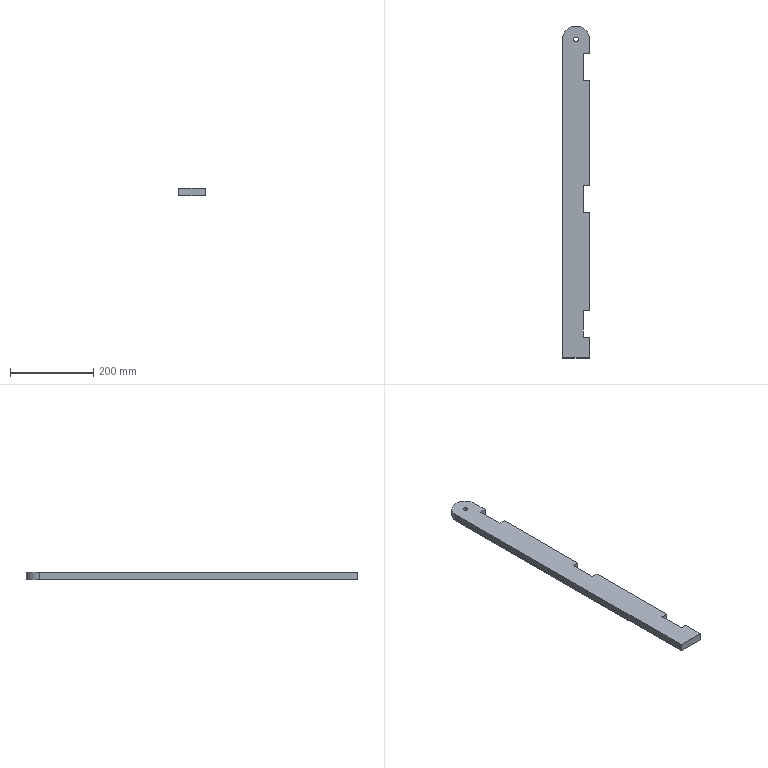Part | STEP file | Superstructure_3_1 | 1 solid | 19 faces | box 65 x 800 x 18 mm | volume 873479 mm3 | plane 17 | cylinder 2 | commonest cylinder face diameters 11 x1 65 x1
STEP:
#1=CARTESIAN_POINT('',(0.,0.,0.));
#2=DIRECTION('',(0.,0.,1.));
#3=DIRECTION('',(1.,0.,0.));
#4=AXIS2_PLACEMENT_3D('',#1,#2,#3);
#5=CARTESIAN_POINT('',(32.5,-35.,-9.));
#6=VERTEX_POINT('',#5);
#7=CARTESIAN_POINT('',(32.5,-35.,9.));
#8=VERTEX_POINT('',#7);
#9=CARTESIAN_POINT('',(32.5,-35.,-9.));
#10=DIRECTION('',(0.,0.,1.));
#11=VECTOR('',#10,1.);
#12=LINE('',#9,#11);
#13=CARTESIAN_POINT('',(32.5,-35.,-9.));
#14=DIRECTION('',(-1.,0.,0.));
#15=DIRECTION('',(0.,1.,0.));
#16=AXIS2_PLACEMENT_3D('',#13,#14,#15);
#17=PLANE('',#16);
#18=CARTESIAN_POINT('',(0.,0.));
#19=DIRECTION('',(0.,-1.));
#20=VECTOR('',#19,1.);
#21=LINE('',#18,#20);
#22=(GEOMETRIC_REPRESENTATION_CONTEXT(2)PARAMETRIC_REPRESENTATION_CONTEXT()REPRESENTATION_CONTEXT('',''));
#23=DEFINITIONAL_REPRESENTATION('',(#21),#22);
#24=PCURVE('',#17,#23);
#25=CARTESIAN_POINT('',(32.5,-35.,-9.));
#26=DIRECTION('',(0.,-1.,0.));
#27=DIRECTION('',(-1.,0.,0.));
#28=AXIS2_PLACEMENT_3D('',#25,#26,#27);
#29=PLANE('',#28);
#30=CARTESIAN_POINT('',(0.,0.));
#31=DIRECTION('',(0.,-1.));
#32=VECTOR('',#31,1.);
#33=LINE('',#30,#32);
#34=(GEOMETRIC_REPRESENTATION_CONTEXT(2)PARAMETRIC_REPRESENTATION_CONTEXT()REPRESENTATION_CONTEXT('',''));
#35=DEFINITIONAL_REPRESENTATION('',(#33),#34);
#36=PCURVE('',#29,#35);
#37=SURFACE_CURVE('',#12,(#24,#36),.PCURVE_S1.);
#38=EDGE_CURVE('',#6,#8,#37,.T.);
#39=ORIENTED_EDGE('',*,*,#38,.T.);
#40=CARTESIAN_POINT('',(32.5,0.,9.));
#41=VERTEX_POINT('',#40);
#42=CARTESIAN_POINT('',(32.5,-35.,9.));
#43=DIRECTION('',(0.,1.,0.));
#44=VECTOR('',#43,1.);
#45=LINE('',#42,#44);
#46=CARTESIAN_POINT('',(0.,-18.));
#47=DIRECTION('',(1.,0.));
#48=VECTOR('',#47,1.);
#49=LINE('',#46,#48);
#50=(GEOMETRIC_REPRESENTATION_CONTEXT(2)PARAMETRIC_REPRESENTATION_CONTEXT()REPRESENTATION_CONTEXT('',''));
#51=DEFINITIONAL_REPRESENTATION('',(#49),#50);
#52=PCURVE('',#17,#51);
#53=CARTESIAN_POINT('',(-0.3717,-369.588,9.));
#54=DIRECTION('',(0.,0.,1.));
#55=DIRECTION('',(1.,0.,0.));
#56=AXIS2_PLACEMENT_3D('',#53,#54,#55);
#57=PLANE('',#56);
#58=CARTESIAN_POINT('',(32.872,334.588));
#59=DIRECTION('',(0.,1.));
#60=VECTOR('',#59,1.);
#61=LINE('',#58,#60);
#62=(GEOMETRIC_REPRESENTATION_CONTEXT(2)PARAMETRIC_REPRESENTATION_CONTEXT()REPRESENTATION_CONTEXT('',''));
#63=DEFINITIONAL_REPRESENTATION('',(#61),#62);
#64=PCURVE('',#57,#63);
#65=SURFACE_CURVE('',#45,(#52,#64),.PCURVE_S1.);
#66=EDGE_CURVE('',#8,#41,#65,.T.);
#67=ORIENTED_EDGE('',*,*,#66,.T.);
#68=CARTESIAN_POINT('',(32.5,0.,-9.));
#69=VERTEX_POINT('',#68);
#70=CARTESIAN_POINT('',(32.5,0.,-9.));
#71=DIRECTION('',(0.,0.,1.));
#72=VECTOR('',#71,1.);
#73=LINE('',#70,#72);
#74=CARTESIAN_POINT('',(35.,0.));
#75=DIRECTION('',(0.,-1.));
#76=VECTOR('',#75,1.);
#77=LINE('',#74,#76);
#78=(GEOMETRIC_REPRESENTATION_CONTEXT(2)PARAMETRIC_REPRESENTATION_CONTEXT()REPRESENTATION_CONTEXT('',''));
#79=DEFINITIONAL_REPRESENTATION('',(#77),#78);
#80=PCURVE('',#17,#79);
#81=CARTESIAN_POINT('',(0.,0.,-9.));
#82=DIRECTION('',(0.,0.,-1.));
#83=DIRECTION('',(1.,0.,0.));
#84=AXIS2_PLACEMENT_3D('',#81,#82,#83);
#85=CYLINDRICAL_SURFACE('',#84,32.5);
#86=CARTESIAN_POINT('',(6.283,0.));
#87=DIRECTION('',(0.,-1.));
#88=VECTOR('',#87,1.);
#89=LINE('',#86,#88);
#90=(GEOMETRIC_REPRESENTATION_CONTEXT(2)PARAMETRIC_REPRESENTATION_CONTEXT()REPRESENTATION_CONTEXT('',''));
#91=DEFINITIONAL_REPRESENTATION('',(#89),#90);
#92=PCURVE('',#85,#91);
#93=SURFACE_CURVE('',#73,(#80,#92),.PCURVE_S1.);
#94=EDGE_CURVE('',#69,#41,#93,.T.);
#95=ORIENTED_EDGE('',*,*,#94,.F.);
#96=CARTESIAN_POINT('',(32.5,-35.,-9.));
#97=DIRECTION('',(0.,1.,0.));
#98=VECTOR('',#97,1.);
#99=LINE('',#96,#98);
#100=CARTESIAN_POINT('',(0.,0.));
#101=DIRECTION('',(1.,0.));
#102=VECTOR('',#101,1.);
#103=LINE('',#100,#102);
#104=(GEOMETRIC_REPRESENTATION_CONTEXT(2)PARAMETRIC_REPRESENTATION_CONTEXT()REPRESENTATION_CONTEXT('',''));
#105=DEFINITIONAL_REPRESENTATION('',(#103),#104);
#106=PCURVE('',#17,#105);
#107=CARTESIAN_POINT('',(-0.3717,-369.588,-9.));
#108=DIRECTION('',(0.,0.,1.));
#109=DIRECTION('',(1.,0.,0.));
#110=AXIS2_PLACEMENT_3D('',#107,#108,#109);
#111=PLANE('',#110);
#112=CARTESIAN_POINT('',(32.872,334.588));
#113=DIRECTION('',(0.,1.));
#114=VECTOR('',#113,1.);
#115=LINE('',#112,#114);
#116=(GEOMETRIC_REPRESENTATION_CONTEXT(2)PARAMETRIC_REPRESENTATION_CONTEXT()REPRESENTATION_CONTEXT('',''));
#117=DEFINITIONAL_REPRESENTATION('',(#115),#116);
#118=PCURVE('',#111,#117);
#119=SURFACE_CURVE('',#99,(#106,#118),.PCURVE_S1.);
#120=EDGE_CURVE('',#6,#69,#119,.T.);
#121=ORIENTED_EDGE('',*,*,#120,.F.);
#122=EDGE_LOOP('',(#39,#67,#95,#121));
#123=FACE_BOUND('',#122,.F.);
#124=ADVANCED_FACE('',(#123),#17,.F.);
#125=CARTESIAN_POINT('',(-32.5,0.,-9.));
#126=VERTEX_POINT('',#125);
#127=CARTESIAN_POINT('',(0.,0.,-9.));
#128=DIRECTION('',(0.,0.,1.));
#129=DIRECTION('',(1.,0.,0.));
#130=AXIS2_PLACEMENT_3D('',#127,#128,#129);
#131=CIRCLE('',#130,32.5);
#132=CARTESIAN_POINT('',(6.283,0.));
#133=DIRECTION('',(-1.,0.));
#134=VECTOR('',#133,1.);
#135=LINE('',#132,#134);
#136=(GEOMETRIC_REPRESENTATION_CONTEXT(2)PARAMETRIC_REPRESENTATION_CONTEXT()REPRESENTATION_CONTEXT('',''));
#137=DEFINITIONAL_REPRESENTATION('',(#135),#136);
#138=PCURVE('',#85,#137);
#139=CARTESIAN_POINT('',(0.3717,369.588));
#140=DIRECTION('',(1.,0.));
#141=AXIS2_PLACEMENT_2D('',#139,#140);
#142=CIRCLE('',#141,32.5);
#143=(GEOMETRIC_REPRESENTATION_CONTEXT(2)PARAMETRIC_REPRESENTATION_CONTEXT()REPRESENTATION_CONTEXT('',''));
#144=DEFINITIONAL_REPRESENTATION('',(#142),#143);
#145=PCURVE('',#111,#144);
#146=SURFACE_CURVE('',#131,(#138,#145),.PCURVE_S1.);
#147=EDGE_CURVE('',#69,#126,#146,.T.);
#148=ORIENTED_EDGE('',*,*,#147,.T.);
#149=CARTESIAN_POINT('',(-32.5,0.,9.));
#150=VERTEX_POINT('',#149);
#151=CARTESIAN_POINT('',(-32.5,0.,-9.));
#152=DIRECTION('',(0.,0.,1.));
#153=VECTOR('',#152,1.);
#154=LINE('',#151,#153);
#155=CARTESIAN_POINT('',(3.142,0.));
#156=DIRECTION('',(0.,-1.));
#157=VECTOR('',#156,1.);
#158=LINE('',#155,#157);
#159=(GEOMETRIC_REPRESENTATION_CONTEXT(2)PARAMETRIC_REPRESENTATION_CONTEXT()REPRESENTATION_CONTEXT('',''));
#160=DEFINITIONAL_REPRESENTATION('',(#158),#159);
#161=PCURVE('',#85,#160);
#162=CARTESIAN_POINT('',(-32.5,0.,-9.));
#163=DIRECTION('',(1.,0.,0.));
#164=DIRECTION('',(0.,-1.,0.));
#165=AXIS2_PLACEMENT_3D('',#162,#163,#164);
#166=PLANE('',#165);
#167=CARTESIAN_POINT('',(0.,0.));
#168=DIRECTION('',(0.,-1.));
#169=VECTOR('',#168,1.);
#170=LINE('',#167,#169);
#171=(GEOMETRIC_REPRESENTATION_CONTEXT(2)PARAMETRIC_REPRESENTATION_CONTEXT()REPRESENTATION_CONTEXT('',''));
#172=DEFINITIONAL_REPRESENTATION('',(#170),#171);
#173=PCURVE('',#166,#172);
#174=SURFACE_CURVE('',#154,(#161,#173),.PCURVE_S1.);
#175=EDGE_CURVE('',#126,#150,#174,.T.);
#176=ORIENTED_EDGE('',*,*,#175,.T.);
#177=CARTESIAN_POINT('',(0.,0.,9.));
#178=DIRECTION('',(0.,0.,1.));
#179=DIRECTION('',(1.,0.,0.));
#180=AXIS2_PLACEMENT_3D('',#177,#178,#179);
#181=CIRCLE('',#180,32.5);
#182=CARTESIAN_POINT('',(6.283,-18.));
#183=DIRECTION('',(-1.,0.));
#184=VECTOR('',#183,1.);
#185=LINE('',#182,#184);
#186=(GEOMETRIC_REPRESENTATION_CONTEXT(2)PARAMETRIC_REPRESENTATION_CONTEXT()REPRESENTATION_CONTEXT('',''));
#187=DEFINITIONAL_REPRESENTATION('',(#185),#186);
#188=PCURVE('',#85,#187);
#189=CARTESIAN_POINT('',(0.3717,369.588));
#190=DIRECTION('',(1.,0.));
#191=AXIS2_PLACEMENT_2D('',#189,#190);
#192=CIRCLE('',#191,32.5);
#193=(GEOMETRIC_REPRESENTATION_CONTEXT(2)PARAMETRIC_REPRESENTATION_CONTEXT()REPRESENTATION_CONTEXT('',''));
#194=DEFINITIONAL_REPRESENTATION('',(#192),#193);
#195=PCURVE('',#57,#194);
#196=SURFACE_CURVE('',#181,(#188,#195),.PCURVE_S1.);
#197=EDGE_CURVE('',#41,#150,#196,.T.);
#198=ORIENTED_EDGE('',*,*,#197,.F.);
#199=ORIENTED_EDGE('',*,*,#94,.F.);
#200=EDGE_LOOP('',(#148,#176,#198,#199));
#201=FACE_BOUND('',#200,.T.);
#202=ADVANCED_FACE('',(#201),#85,.T.);
#203=ORIENTED_EDGE('',*,*,#175,.T.);
#204=CARTESIAN_POINT('',(-32.5,-767.5,9.));
#205=VERTEX_POINT('',#204);
#206=CARTESIAN_POINT('',(-32.5,0.,9.));
#207=DIRECTION('',(0.,-1.,0.));
#208=VECTOR('',#207,1.);
#209=LINE('',#206,#208);
#210=CARTESIAN_POINT('',(0.,-18.));
#211=DIRECTION('',(1.,0.));
#212=VECTOR('',#211,1.);
#213=LINE('',#210,#212);
#214=(GEOMETRIC_REPRESENTATION_CONTEXT(2)PARAMETRIC_REPRESENTATION_CONTEXT()REPRESENTATION_CONTEXT('',''));
#215=DEFINITIONAL_REPRESENTATION('',(#213),#214);
#216=PCURVE('',#166,#215);
#217=CARTESIAN_POINT('',(-32.128,369.588));
#218=DIRECTION('',(0.,-1.));
#219=VECTOR('',#218,1.);
#220=LINE('',#217,#219);
#221=(GEOMETRIC_REPRESENTATION_CONTEXT(2)PARAMETRIC_REPRESENTATION_CONTEXT()REPRESENTATION_CONTEXT('',''));
#222=DEFINITIONAL_REPRESENTATION('',(#220),#221);
#223=PCURVE('',#57,#222);
#224=SURFACE_CURVE('',#209,(#216,#223),.PCURVE_S1.);
#225=EDGE_CURVE('',#150,#205,#224,.T.);
#226=ORIENTED_EDGE('',*,*,#225,.T.);
#227=CARTESIAN_POINT('',(-32.5,-767.5,-9.));
#228=VERTEX_POINT('',#227);
#229=CARTESIAN_POINT('',(-32.5,-767.5,-9.));
#230=DIRECTION('',(0.,0.,1.));
#231=VECTOR('',#230,1.);
#232=LINE('',#229,#231);
#233=CARTESIAN_POINT('',(767.5,0.));
#234=DIRECTION('',(0.,-1.));
#235=VECTOR('',#234,1.);
#236=LINE('',#233,#235);
#237=(GEOMETRIC_REPRESENTATION_CONTEXT(2)PARAMETRIC_REPRESENTATION_CONTEXT()REPRESENTATION_CONTEXT('',''));
#238=DEFINITIONAL_REPRESENTATION('',(#236),#237);
#239=PCURVE('',#166,#238);
#240=CARTESIAN_POINT('',(-32.5,-767.5,-9.));
#241=DIRECTION('',(0.,1.,0.));
#242=DIRECTION('',(1.,0.,0.));
#243=AXIS2_PLACEMENT_3D('',#240,#241,#242);
#244=PLANE('',#243);
#245=CARTESIAN_POINT('',(0.,0.));
#246=DIRECTION('',(0.,-1.));
#247=VECTOR('',#246,1.);
#248=LINE('',#245,#247);
#249=(GEOMETRIC_REPRESENTATION_CONTEXT(2)PARAMETRIC_REPRESENTATION_CONTEXT()REPRESENTATION_CONTEXT('',''));
#250=DEFINITIONAL_REPRESENTATION('',(#248),#249);
#251=PCURVE('',#244,#250);
#252=SURFACE_CURVE('',#232,(#239,#251),.PCURVE_S1.);
#253=EDGE_CURVE('',#228,#205,#252,.T.);
#254=ORIENTED_EDGE('',*,*,#253,.F.);
#255=CARTESIAN_POINT('',(-32.5,0.,-9.));
#256=DIRECTION('',(0.,-1.,0.));
#257=VECTOR('',#256,1.);
#258=LINE('',#255,#257);
#259=CARTESIAN_POINT('',(0.,0.));
#260=DIRECTION('',(1.,0.));
#261=VECTOR('',#260,1.);
#262=LINE('',#259,#261);
#263=(GEOMETRIC_REPRESENTATION_CONTEXT(2)PARAMETRIC_REPRESENTATION_CONTEXT()REPRESENTATION_CONTEXT('',''));
#264=DEFINITIONAL_REPRESENTATION('',(#262),#263);
#265=PCURVE('',#166,#264);
#266=CARTESIAN_POINT('',(-32.128,369.588));
#267=DIRECTION('',(0.,-1.));
#268=VECTOR('',#267,1.);
#269=LINE('',#266,#268);
#270=(GEOMETRIC_REPRESENTATION_CONTEXT(2)PARAMETRIC_REPRESENTATION_CONTEXT()REPRESENTATION_CONTEXT('',''));
#271=DEFINITIONAL_REPRESENTATION('',(#269),#270);
#272=PCURVE('',#111,#271);
#273=SURFACE_CURVE('',#258,(#265,#272),.PCURVE_S1.);
#274=EDGE_CURVE('',#126,#228,#273,.T.);
#275=ORIENTED_EDGE('',*,*,#274,.F.);
#276=EDGE_LOOP('',(#203,#226,#254,#275));
#277=FACE_BOUND('',#276,.F.);
#278=ADVANCED_FACE('',(#277),#166,.F.);
#279=ORIENTED_EDGE('',*,*,#253,.T.);
#280=CARTESIAN_POINT('',(32.5,-767.5,9.));
#281=VERTEX_POINT('',#280);
#282=CARTESIAN_POINT('',(-32.5,-767.5,9.));
#283=DIRECTION('',(1.,0.,0.));
#284=VECTOR('',#283,1.);
#285=LINE('',#282,#284);
#286=CARTESIAN_POINT('',(0.,-18.));
#287=DIRECTION('',(1.,0.));
#288=VECTOR('',#287,1.);
#289=LINE('',#286,#288);
#290=(GEOMETRIC_REPRESENTATION_CONTEXT(2)PARAMETRIC_REPRESENTATION_CONTEXT()REPRESENTATION_CONTEXT('',''));
#291=DEFINITIONAL_REPRESENTATION('',(#289),#290);
#292=PCURVE('',#244,#291);
#293=CARTESIAN_POINT('',(-32.128,-397.912));
#294=DIRECTION('',(1.,0.));
#295=VECTOR('',#294,1.);
#296=LINE('',#293,#295);
#297=(GEOMETRIC_REPRESENTATION_CONTEXT(2)PARAMETRIC_REPRESENTATION_CONTEXT()REPRESENTATION_CONTEXT('',''));
#298=DEFINITIONAL_REPRESENTATION('',(#296),#297);
#299=PCURVE('',#57,#298);
#300=SURFACE_CURVE('',#285,(#292,#299),.PCURVE_S1.);
#301=EDGE_CURVE('',#205,#281,#300,.T.);
#302=ORIENTED_EDGE('',*,*,#301,.T.);
#303=CARTESIAN_POINT('',(32.5,-767.5,-9.));
#304=VERTEX_POINT('',#303);
#305=CARTESIAN_POINT('',(32.5,-767.5,-9.));
#306=DIRECTION('',(0.,0.,1.));
#307=VECTOR('',#306,1.);
#308=LINE('',#305,#307);
#309=CARTESIAN_POINT('',(65.,0.));
#310=DIRECTION('',(0.,-1.));
#311=VECTOR('',#310,1.);
#312=LINE('',#309,#311);
#313=(GEOMETRIC_REPRESENTATION_CONTEXT(2)PARAMETRIC_REPRESENTATION_CONTEXT()REPRESENTATION_CONTEXT('',''));
#314=DEFINITIONAL_REPRESENTATION('',(#312),#313);
#315=PCURVE('',#244,#314);
#316=CARTESIAN_POINT('',(32.5,-767.5,-9.));
#317=DIRECTION('',(-1.,0.,0.));
#318=DIRECTION('',(0.,1.,0.));
#319=AXIS2_PLACEMENT_3D('',#316,#317,#318);
#320=PLANE('',#319);
#321=CARTESIAN_POINT('',(0.,0.));
#322=DIRECTION('',(0.,-1.));
#323=VECTOR('',#322,1.);
#324=LINE('',#321,#323);
#325=(GEOMETRIC_REPRESENTATION_CONTEXT(2)PARAMETRIC_REPRESENTATION_CONTEXT()REPRESENTATION_CONTEXT('',''));
#326=DEFINITIONAL_REPRESENTATION('',(#324),#325);
#327=PCURVE('',#320,#326);
#328=SURFACE_CURVE('',#308,(#315,#327),.PCURVE_S1.);
#329=EDGE_CURVE('',#304,#281,#328,.T.);
#330=ORIENTED_EDGE('',*,*,#329,.F.);
#331=CARTESIAN_POINT('',(-32.5,-767.5,-9.));
#332=DIRECTION('',(1.,0.,0.));
#333=VECTOR('',#332,1.);
#334=LINE('',#331,#333);
#335=CARTESIAN_POINT('',(0.,0.));
#336=DIRECTION('',(1.,0.));
#337=VECTOR('',#336,1.);
#338=LINE('',#335,#337);
#339=(GEOMETRIC_REPRESENTATION_CONTEXT(2)PARAMETRIC_REPRESENTATION_CONTEXT()REPRESENTATION_CONTEXT('',''));
#340=DEFINITIONAL_REPRESENTATION('',(#338),#339);
#341=PCURVE('',#244,#340);
#342=CARTESIAN_POINT('',(-32.128,-397.912));
#343=DIRECTION('',(1.,0.));
#344=VECTOR('',#343,1.);
#345=LINE('',#342,#344);
#346=(GEOMETRIC_REPRESENTATION_CONTEXT(2)PARAMETRIC_REPRESENTATION_CONTEXT()REPRESENTATION_CONTEXT('',''));
#347=DEFINITIONAL_REPRESENTATION('',(#345),#346);
#348=PCURVE('',#111,#347);
#349=SURFACE_CURVE('',#334,(#341,#348),.PCURVE_S1.);
#350=EDGE_CURVE('',#228,#304,#349,.T.);
#351=ORIENTED_EDGE('',*,*,#350,.F.);
#352=EDGE_LOOP('',(#279,#302,#330,#351));
#353=FACE_BOUND('',#352,.F.);
#354=ADVANCED_FACE('',(#353),#244,.F.);
#355=ORIENTED_EDGE('',*,*,#329,.T.);
#356=CARTESIAN_POINT('',(32.5,-717.5,9.));
#357=VERTEX_POINT('',#356);
#358=CARTESIAN_POINT('',(32.5,-767.5,9.));
#359=DIRECTION('',(0.,1.,0.));
#360=VECTOR('',#359,1.);
#361=LINE('',#358,#360);
#362=CARTESIAN_POINT('',(0.,-18.));
#363=DIRECTION('',(1.,0.));
#364=VECTOR('',#363,1.);
#365=LINE('',#362,#364);
#366=(GEOMETRIC_REPRESENTATION_CONTEXT(2)PARAMETRIC_REPRESENTATION_CONTEXT()REPRESENTATION_CONTEXT('',''));
#367=DEFINITIONAL_REPRESENTATION('',(#365),#366);
#368=PCURVE('',#320,#367);
#369=CARTESIAN_POINT('',(32.872,-397.912));
#370=DIRECTION('',(0.,1.));
#371=VECTOR('',#370,1.);
#372=LINE('',#369,#371);
#373=(GEOMETRIC_REPRESENTATION_CONTEXT(2)PARAMETRIC_REPRESENTATION_CONTEXT()REPRESENTATION_CONTEXT('',''));
#374=DEFINITIONAL_REPRESENTATION('',(#372),#373);
#375=PCURVE('',#57,#374);
#376=SURFACE_CURVE('',#361,(#368,#375),.PCURVE_S1.);
#377=EDGE_CURVE('',#281,#357,#376,.T.);
#378=ORIENTED_EDGE('',*,*,#377,.T.);
#379=CARTESIAN_POINT('',(32.5,-717.5,-9.));
#380=VERTEX_POINT('',#379);
#381=CARTESIAN_POINT('',(32.5,-717.5,-9.));
#382=DIRECTION('',(0.,0.,1.));
#383=VECTOR('',#382,1.);
#384=LINE('',#381,#383);
#385=CARTESIAN_POINT('',(50.,0.));
#386=DIRECTION('',(0.,-1.));
#387=VECTOR('',#386,1.);
#388=LINE('',#385,#387);
#389=(GEOMETRIC_REPRESENTATION_CONTEXT(2)PARAMETRIC_REPRESENTATION_CONTEXT()REPRESENTATION_CONTEXT('',''));
#390=DEFINITIONAL_REPRESENTATION('',(#388),#389);
#391=PCURVE('',#320,#390);
#392=CARTESIAN_POINT('',(32.5,-717.5,-9.));
#393=DIRECTION('',(0.,-1.,0.));
#394=DIRECTION('',(-1.,0.,0.));
#395=AXIS2_PLACEMENT_3D('',#392,#393,#394);
#396=PLANE('',#395);
#397=CARTESIAN_POINT('',(0.,0.));
#398=DIRECTION('',(0.,-1.));
#399=VECTOR('',#398,1.);
#400=LINE('',#397,#399);
#401=(GEOMETRIC_REPRESENTATION_CONTEXT(2)PARAMETRIC_REPRESENTATION_CONTEXT()REPRESENTATION_CONTEXT('',''));
#402=DEFINITIONAL_REPRESENTATION('',(#400),#401);
#403=PCURVE('',#396,#402);
#404=SURFACE_CURVE('',#384,(#391,#403),.PCURVE_S1.);
#405=EDGE_CURVE('',#380,#357,#404,.T.);
#406=ORIENTED_EDGE('',*,*,#405,.F.);
#407=CARTESIAN_POINT('',(32.5,-767.5,-9.));
#408=DIRECTION('',(0.,1.,0.));
#409=VECTOR('',#408,1.);
#410=LINE('',#407,#409);
#411=CARTESIAN_POINT('',(0.,0.));
#412=DIRECTION('',(1.,0.));
#413=VECTOR('',#412,1.);
#414=LINE('',#411,#413);
#415=(GEOMETRIC_REPRESENTATION_CONTEXT(2)PARAMETRIC_REPRESENTATION_CONTEXT()REPRESENTATION_CONTEXT('',''));
#416=DEFINITIONAL_REPRESENTATION('',(#414),#415);
#417=PCURVE('',#320,#416);
#418=CARTESIAN_POINT('',(32.872,-397.912));
#419=DIRECTION('',(0.,1.));
#420=VECTOR('',#419,1.);
#421=LINE('',#418,#420);
#422=(GEOMETRIC_REPRESENTATION_CONTEXT(2)PARAMETRIC_REPRESENTATION_CONTEXT()REPRESENTATION_CONTEXT('',''));
#423=DEFINITIONAL_REPRESENTATION('',(#421),#422);
#424=PCURVE('',#111,#423);
#425=SURFACE_CURVE('',#410,(#417,#424),.PCURVE_S1.);
#426=EDGE_CURVE('',#304,#380,#425,.T.);
#427=ORIENTED_EDGE('',*,*,#426,.F.);
#428=EDGE_LOOP('',(#355,#378,#406,#427));
#429=FACE_BOUND('',#428,.F.);
#430=ADVANCED_FACE('',(#429),#320,.F.);
#431=ORIENTED_EDGE('',*,*,#405,.T.);
#432=CARTESIAN_POINT('',(17.5,-717.5,9.));
#433=VERTEX_POINT('',#432);
#434=CARTESIAN_POINT('',(32.5,-717.5,9.));
#435=DIRECTION('',(-1.,0.,0.));
#436=VECTOR('',#435,1.);
#437=LINE('',#434,#436);
#438=CARTESIAN_POINT('',(0.,-18.));
#439=DIRECTION('',(1.,0.));
#440=VECTOR('',#439,1.);
#441=LINE('',#438,#440);
#442=(GEOMETRIC_REPRESENTATION_CONTEXT(2)PARAMETRIC_REPRESENTATION_CONTEXT()REPRESENTATION_CONTEXT('',''));
#443=DEFINITIONAL_REPRESENTATION('',(#441),#442);
#444=PCURVE('',#396,#443);
#445=CARTESIAN_POINT('',(32.872,-347.912));
#446=DIRECTION('',(-1.,0.));
#447=VECTOR('',#446,1.);
#448=LINE('',#445,#447);
#449=(GEOMETRIC_REPRESENTATION_CONTEXT(2)PARAMETRIC_REPRESENTATION_CONTEXT()REPRESENTATION_CONTEXT('',''));
#450=DEFINITIONAL_REPRESENTATION('',(#448),#449);
#451=PCURVE('',#57,#450);
#452=SURFACE_CURVE('',#437,(#444,#451),.PCURVE_S1.);
#453=EDGE_CURVE('',#357,#433,#452,.T.);
#454=ORIENTED_EDGE('',*,*,#453,.T.);
#455=CARTESIAN_POINT('',(17.5,-717.5,-9.));
#456=VERTEX_POINT('',#455);
#457=CARTESIAN_POINT('',(17.5,-717.5,-9.));
#458=DIRECTION('',(0.,0.,1.));
#459=VECTOR('',#458,1.);
#460=LINE('',#457,#459);
#461=CARTESIAN_POINT('',(15.,0.));
#462=DIRECTION('',(0.,-1.));
#463=VECTOR('',#462,1.);
#464=LINE('',#461,#463);
#465=(GEOMETRIC_REPRESENTATION_CONTEXT(2)PARAMETRIC_REPRESENTATION_CONTEXT()REPRESENTATION_CONTEXT('',''));
#466=DEFINITIONAL_REPRESENTATION('',(#464),#465);
#467=PCURVE('',#396,#466);
#468=CARTESIAN_POINT('',(17.5,-717.5,-9.));
#469=DIRECTION('',(-1.,0.,0.));
#470=DIRECTION('',(0.,1.,0.));
#471=AXIS2_PLACEMENT_3D('',#468,#469,#470);
#472=PLANE('',#471);
#473=CARTESIAN_POINT('',(0.,0.));
#474=DIRECTION('',(0.,-1.));
#475=VECTOR('',#474,1.);
#476=LINE('',#473,#475);
#477=(GEOMETRIC_REPRESENTATION_CONTEXT(2)PARAMETRIC_REPRESENTATION_CONTEXT()REPRESENTATION_CONTEXT('',''));
#478=DEFINITIONAL_REPRESENTATION('',(#476),#477);
#479=PCURVE('',#472,#478);
#480=SURFACE_CURVE('',#460,(#467,#479),.PCURVE_S1.);
#481=EDGE_CURVE('',#456,#433,#480,.T.);
#482=ORIENTED_EDGE('',*,*,#481,.F.);
#483=CARTESIAN_POINT('',(32.5,-717.5,-9.));
#484=DIRECTION('',(-1.,0.,0.));
#485=VECTOR('',#484,1.);
#486=LINE('',#483,#485);
#487=CARTESIAN_POINT('',(0.,0.));
#488=DIRECTION('',(1.,0.));
#489=VECTOR('',#488,1.);
#490=LINE('',#487,#489);
#491=(GEOMETRIC_REPRESENTATION_CONTEXT(2)PARAMETRIC_REPRESENTATION_CONTEXT()REPRESENTATION_CONTEXT('',''));
#492=DEFINITIONAL_REPRESENTATION('',(#490),#491);
#493=PCURVE('',#396,#492);
#494=CARTESIAN_POINT('',(32.872,-347.912));
#495=DIRECTION('',(-1.,0.));
#496=VECTOR('',#495,1.);
#497=LINE('',#494,#496);
#498=(GEOMETRIC_REPRESENTATION_CONTEXT(2)PARAMETRIC_REPRESENTATION_CONTEXT()REPRESENTATION_CONTEXT('',''));
#499=DEFINITIONAL_REPRESENTATION('',(#497),#498);
#500=PCURVE('',#111,#499);
#501=SURFACE_CURVE('',#486,(#493,#500),.PCURVE_S1.);
#502=EDGE_CURVE('',#380,#456,#501,.T.);
#503=ORIENTED_EDGE('',*,*,#502,.F.);
#504=EDGE_LOOP('',(#431,#454,#482,#503));
#505=FACE_BOUND('',#504,.F.);
#506=ADVANCED_FACE('',(#505),#396,.F.);
#507=ORIENTED_EDGE('',*,*,#481,.T.);
#508=CARTESIAN_POINT('',(17.5,-652.5,9.));
#509=VERTEX_POINT('',#508);
#510=CARTESIAN_POINT('',(17.5,-717.5,9.));
#511=DIRECTION('',(0.,1.,0.));
#512=VECTOR('',#511,1.);
#513=LINE('',#510,#512);
#514=CARTESIAN_POINT('',(0.,-18.));
#515=DIRECTION('',(1.,0.));
#516=VECTOR('',#515,1.);
#517=LINE('',#514,#516);
#518=(GEOMETRIC_REPRESENTATION_CONTEXT(2)PARAMETRIC_REPRESENTATION_CONTEXT()REPRESENTATION_CONTEXT('',''));
#519=DEFINITIONAL_REPRESENTATION('',(#517),#518);
#520=PCURVE('',#472,#519);
#521=CARTESIAN_POINT('',(17.872,-347.912));
#522=DIRECTION('',(0.,1.));
#523=VECTOR('',#522,1.);
#524=LINE('',#521,#523);
#525=(GEOMETRIC_REPRESENTATION_CONTEXT(2)PARAMETRIC_REPRESENTATION_CONTEXT()REPRESENTATION_CONTEXT('',''));
#526=DEFINITIONAL_REPRESENTATION('',(#524),#525);
#527=PCURVE('',#57,#526);
#528=SURFACE_CURVE('',#513,(#520,#527),.PCURVE_S1.);
#529=EDGE_CURVE('',#433,#509,#528,.T.);
#530=ORIENTED_EDGE('',*,*,#529,.T.);
#531=CARTESIAN_POINT('',(17.5,-652.5,-9.));
#532=VERTEX_POINT('',#531);
#533=CARTESIAN_POINT('',(17.5,-652.5,-9.));
#534=DIRECTION('',(0.,0.,1.));
#535=VECTOR('',#534,1.);
#536=LINE('',#533,#535);
#537=CARTESIAN_POINT('',(65.,0.));
#538=DIRECTION('',(0.,-1.));
#539=VECTOR('',#538,1.);
#540=LINE('',#537,#539);
#541=(GEOMETRIC_REPRESENTATION_CONTEXT(2)PARAMETRIC_REPRESENTATION_CONTEXT()REPRESENTATION_CONTEXT('',''));
#542=DEFINITIONAL_REPRESENTATION('',(#540),#541);
#543=PCURVE('',#472,#542);
#544=CARTESIAN_POINT('',(17.5,-652.5,-9.));
#545=DIRECTION('',(0.,1.,0.));
#546=DIRECTION('',(1.,0.,0.));
#547=AXIS2_PLACEMENT_3D('',#544,#545,#546);
#548=PLANE('',#547);
#549=CARTESIAN_POINT('',(0.,0.));
#550=DIRECTION('',(0.,-1.));
#551=VECTOR('',#550,1.);
#552=LINE('',#549,#551);
#553=(GEOMETRIC_REPRESENTATION_CONTEXT(2)PARAMETRIC_REPRESENTATION_CONTEXT()REPRESENTATION_CONTEXT('',''));
#554=DEFINITIONAL_REPRESENTATION('',(#552),#553);
#555=PCURVE('',#548,#554);
#556=SURFACE_CURVE('',#536,(#543,#555),.PCURVE_S1.);
#557=EDGE_CURVE('',#532,#509,#556,.T.);
#558=ORIENTED_EDGE('',*,*,#557,.F.);
#559=CARTESIAN_POINT('',(17.5,-717.5,-9.));
#560=DIRECTION('',(0.,1.,0.));
#561=VECTOR('',#560,1.);
#562=LINE('',#559,#561);
#563=CARTESIAN_POINT('',(0.,0.));
#564=DIRECTION('',(1.,0.));
#565=VECTOR('',#564,1.);
#566=LINE('',#563,#565);
#567=(GEOMETRIC_REPRESENTATION_CONTEXT(2)PARAMETRIC_REPRESENTATION_CONTEXT()REPRESENTATION_CONTEXT('',''));
#568=DEFINITIONAL_REPRESENTATION('',(#566),#567);
#569=PCURVE('',#472,#568);
#570=CARTESIAN_POINT('',(17.872,-347.912));
#571=DIRECTION('',(0.,1.));
#572=VECTOR('',#571,1.);
#573=LINE('',#570,#572);
#574=(GEOMETRIC_REPRESENTATION_CONTEXT(2)PARAMETRIC_REPRESENTATION_CONTEXT()REPRESENTATION_CONTEXT('',''));
#575=DEFINITIONAL_REPRESENTATION('',(#573),#574);
#576=PCURVE('',#111,#575);
#577=SURFACE_CURVE('',#562,(#569,#576),.PCURVE_S1.);
#578=EDGE_CURVE('',#456,#532,#577,.T.);
#579=ORIENTED_EDGE('',*,*,#578,.F.);
#580=EDGE_LOOP('',(#507,#530,#558,#579));
#581=FACE_BOUND('',#580,.F.);
#582=ADVANCED_FACE('',(#581),#472,.F.);
#583=ORIENTED_EDGE('',*,*,#557,.T.);
#584=CARTESIAN_POINT('',(32.5,-652.5,9.));
#585=VERTEX_POINT('',#584);
#586=CARTESIAN_POINT('',(17.5,-652.5,9.));
#587=DIRECTION('',(1.,0.,0.));
#588=VECTOR('',#587,1.);
#589=LINE('',#586,#588);
#590=CARTESIAN_POINT('',(0.,-18.));
#591=DIRECTION('',(1.,0.));
#592=VECTOR('',#591,1.);
#593=LINE('',#590,#592);
#594=(GEOMETRIC_REPRESENTATION_CONTEXT(2)PARAMETRIC_REPRESENTATION_CONTEXT()REPRESENTATION_CONTEXT('',''));
#595=DEFINITIONAL_REPRESENTATION('',(#593),#594);
#596=PCURVE('',#548,#595);
#597=CARTESIAN_POINT('',(17.872,-282.912));
#598=DIRECTION('',(1.,0.));
#599=VECTOR('',#598,1.);
#600=LINE('',#597,#599);
#601=(GEOMETRIC_REPRESENTATION_CONTEXT(2)PARAMETRIC_REPRESENTATION_CONTEXT()REPRESENTATION_CONTEXT('',''));
#602=DEFINITIONAL_REPRESENTATION('',(#600),#601);
#603=PCURVE('',#57,#602);
#604=SURFACE_CURVE('',#589,(#596,#603),.PCURVE_S1.);
#605=EDGE_CURVE('',#509,#585,#604,.T.);
#606=ORIENTED_EDGE('',*,*,#605,.T.);
#607=CARTESIAN_POINT('',(32.5,-652.5,-9.));
#608=VERTEX_POINT('',#607);
#609=CARTESIAN_POINT('',(32.5,-652.5,-9.));
#610=DIRECTION('',(0.,0.,1.));
#611=VECTOR('',#610,1.);
#612=LINE('',#609,#611);
#613=CARTESIAN_POINT('',(15.,0.));
#614=DIRECTION('',(0.,-1.));
#615=VECTOR('',#614,1.);
#616=LINE('',#613,#615);
#617=(GEOMETRIC_REPRESENTATION_CONTEXT(2)PARAMETRIC_REPRESENTATION_CONTEXT()REPRESENTATION_CONTEXT('',''));
#618=DEFINITIONAL_REPRESENTATION('',(#616),#617);
#619=PCURVE('',#548,#618);
#620=CARTESIAN_POINT('',(32.5,-652.5,-9.));
#621=DIRECTION('',(-1.,0.,0.));
#622=DIRECTION('',(0.,1.,0.));
#623=AXIS2_PLACEMENT_3D('',#620,#621,#622);
#624=PLANE('',#623);
#625=CARTESIAN_POINT('',(0.,0.));
#626=DIRECTION('',(0.,-1.));
#627=VECTOR('',#626,1.);
#628=LINE('',#625,#627);
#629=(GEOMETRIC_REPRESENTATION_CONTEXT(2)PARAMETRIC_REPRESENTATION_CONTEXT()REPRESENTATION_CONTEXT('',''));
#630=DEFINITIONAL_REPRESENTATION('',(#628),#629);
#631=PCURVE('',#624,#630);
#632=SURFACE_CURVE('',#612,(#619,#631),.PCURVE_S1.);
#633=EDGE_CURVE('',#608,#585,#632,.T.);
#634=ORIENTED_EDGE('',*,*,#633,.F.);
#635=CARTESIAN_POINT('',(17.5,-652.5,-9.));
#636=DIRECTION('',(1.,0.,0.));
#637=VECTOR('',#636,1.);
#638=LINE('',#635,#637);
#639=CARTESIAN_POINT('',(0.,0.));
#640=DIRECTION('',(1.,0.));
#641=VECTOR('',#640,1.);
#642=LINE('',#639,#641);
#643=(GEOMETRIC_REPRESENTATION_CONTEXT(2)PARAMETRIC_REPRESENTATION_CONTEXT()REPRESENTATION_CONTEXT('',''));
#644=DEFINITIONAL_REPRESENTATION('',(#642),#643);
#645=PCURVE('',#548,#644);
#646=CARTESIAN_POINT('',(17.872,-282.912));
#647=DIRECTION('',(1.,0.));
#648=VECTOR('',#647,1.);
#649=LINE('',#646,#648);
#650=(GEOMETRIC_REPRESENTATION_CONTEXT(2)PARAMETRIC_REPRESENTATION_CONTEXT()REPRESENTATION_CONTEXT('',''));
#651=DEFINITIONAL_REPRESENTATION('',(#649),#650);
#652=PCURVE('',#111,#651);
#653=SURFACE_CURVE('',#638,(#645,#652),.PCURVE_S1.);
#654=EDGE_CURVE('',#532,#608,#653,.T.);
#655=ORIENTED_EDGE('',*,*,#654,.F.);
#656=EDGE_LOOP('',(#583,#606,#634,#655));
#657=FACE_BOUND('',#656,.F.);
#658=ADVANCED_FACE('',(#657),#548,.F.);
#659=ORIENTED_EDGE('',*,*,#633,.T.);
#660=CARTESIAN_POINT('',(32.5,-416.25,9.));
#661=VERTEX_POINT('',#660);
#662=CARTESIAN_POINT('',(32.5,-652.5,9.));
#663=DIRECTION('',(0.,1.,0.));
#664=VECTOR('',#663,1.);
#665=LINE('',#662,#664);
#666=CARTESIAN_POINT('',(0.,-18.));
#667=DIRECTION('',(1.,0.));
#668=VECTOR('',#667,1.);
#669=LINE('',#666,#668);
#670=(GEOMETRIC_REPRESENTATION_CONTEXT(2)PARAMETRIC_REPRESENTATION_CONTEXT()REPRESENTATION_CONTEXT('',''));
#671=DEFINITIONAL_REPRESENTATION('',(#669),#670);
#672=PCURVE('',#624,#671);
#673=CARTESIAN_POINT('',(32.872,-282.912));
#674=DIRECTION('',(0.,1.));
#675=VECTOR('',#674,1.);
#676=LINE('',#673,#675);
#677=(GEOMETRIC_REPRESENTATION_CONTEXT(2)PARAMETRIC_REPRESENTATION_CONTEXT()REPRESENTATION_CONTEXT('',''));
#678=DEFINITIONAL_REPRESENTATION('',(#676),#677);
#679=PCURVE('',#57,#678);
#680=SURFACE_CURVE('',#665,(#672,#679),.PCURVE_S1.);
#681=EDGE_CURVE('',#585,#661,#680,.T.);
#682=ORIENTED_EDGE('',*,*,#681,.T.);
#683=CARTESIAN_POINT('',(32.5,-416.25,-9.));
#684=VERTEX_POINT('',#683);
#685=CARTESIAN_POINT('',(32.5,-416.25,-9.));
#686=DIRECTION('',(0.,0.,1.));
#687=VECTOR('',#686,1.);
#688=LINE('',#685,#687);
#689=CARTESIAN_POINT('',(236.25,0.));
#690=DIRECTION('',(0.,-1.));
#691=VECTOR('',#690,1.);
#692=LINE('',#689,#691);
#693=(GEOMETRIC_REPRESENTATION_CONTEXT(2)PARAMETRIC_REPRESENTATION_CONTEXT()REPRESENTATION_CONTEXT('',''));
#694=DEFINITIONAL_REPRESENTATION('',(#692),#693);
#695=PCURVE('',#624,#694);
#696=CARTESIAN_POINT('',(17.5,-416.25,-9.));
#697=DIRECTION('',(0.,1.,0.));
#698=DIRECTION('',(1.,0.,0.));
#699=AXIS2_PLACEMENT_3D('',#696,#697,#698);
#700=PLANE('',#699);
#701=CARTESIAN_POINT('',(15.,0.));
#702=DIRECTION('',(0.,-1.));
#703=VECTOR('',#702,1.);
#704=LINE('',#701,#703);
#705=(GEOMETRIC_REPRESENTATION_CONTEXT(2)PARAMETRIC_REPRESENTATION_CONTEXT()REPRESENTATION_CONTEXT('',''));
#706=DEFINITIONAL_REPRESENTATION('',(#704),#705);
#707=PCURVE('',#700,#706);
#708=SURFACE_CURVE('',#688,(#695,#707),.PCURVE_S1.);
#709=EDGE_CURVE('',#684,#661,#708,.T.);
#710=ORIENTED_EDGE('',*,*,#709,.F.);
#711=CARTESIAN_POINT('',(32.5,-652.5,-9.));
#712=DIRECTION('',(0.,1.,0.));
#713=VECTOR('',#712,1.);
#714=LINE('',#711,#713);
#715=CARTESIAN_POINT('',(0.,0.));
#716=DIRECTION('',(1.,0.));
#717=VECTOR('',#716,1.);
#718=LINE('',#715,#717);
#719=(GEOMETRIC_REPRESENTATION_CONTEXT(2)PARAMETRIC_REPRESENTATION_CONTEXT()REPRESENTATION_CONTEXT('',''));
#720=DEFINITIONAL_REPRESENTATION('',(#718),#719);
#721=PCURVE('',#624,#720);
#722=CARTESIAN_POINT('',(32.872,-282.912));
#723=DIRECTION('',(0.,1.));
#724=VECTOR('',#723,1.);
#725=LINE('',#722,#724);
#726=(GEOMETRIC_REPRESENTATION_CONTEXT(2)PARAMETRIC_REPRESENTATION_CONTEXT()REPRESENTATION_CONTEXT('',''));
#727=DEFINITIONAL_REPRESENTATION('',(#725),#726);
#728=PCURVE('',#111,#727);
#729=SURFACE_CURVE('',#714,(#721,#728),.PCURVE_S1.);
#730=EDGE_CURVE('',#608,#684,#729,.T.);
#731=ORIENTED_EDGE('',*,*,#730,.F.);
#732=EDGE_LOOP('',(#659,#682,#710,#731));
#733=FACE_BOUND('',#732,.F.);
#734=ADVANCED_FACE('',(#733),#624,.F.);
#735=CARTESIAN_POINT('',(17.5,-416.25,-9.));
#736=VERTEX_POINT('',#735);
#737=CARTESIAN_POINT('',(17.5,-416.25,9.));
#738=VERTEX_POINT('',#737);
#739=CARTESIAN_POINT('',(17.5,-416.25,-9.));
#740=DIRECTION('',(0.,0.,1.));
#741=VECTOR('',#740,1.);
#742=LINE('',#739,#741);
#743=CARTESIAN_POINT('',(0.,0.));
#744=DIRECTION('',(0.,-1.));
#745=VECTOR('',#744,1.);
#746=LINE('',#743,#745);
#747=(GEOMETRIC_REPRESENTATION_CONTEXT(2)PARAMETRIC_REPRESENTATION_CONTEXT()REPRESENTATION_CONTEXT('',''));
#748=DEFINITIONAL_REPRESENTATION('',(#746),#747);
#749=PCURVE('',#700,#748);
#750=CARTESIAN_POINT('',(17.5,-351.25,-9.));
#751=DIRECTION('',(1.,0.,0.));
#752=DIRECTION('',(0.,-1.,0.));
#753=AXIS2_PLACEMENT_3D('',#750,#751,#752);
#754=PLANE('',#753);
#755=CARTESIAN_POINT('',(65.,0.));
#756=DIRECTION('',(0.,-1.));
#757=VECTOR('',#756,1.);
#758=LINE('',#755,#757);
#759=(GEOMETRIC_REPRESENTATION_CONTEXT(2)PARAMETRIC_REPRESENTATION_CONTEXT()REPRESENTATION_CONTEXT('',''));
#760=DEFINITIONAL_REPRESENTATION('',(#758),#759);
#761=PCURVE('',#754,#760);
#762=SURFACE_CURVE('',#742,(#749,#761),.PCURVE_S1.);
#763=EDGE_CURVE('',#736,#738,#762,.T.);
#764=ORIENTED_EDGE('',*,*,#763,.T.);
#765=CARTESIAN_POINT('',(17.5,-416.25,9.));
#766=DIRECTION('',(1.,0.,0.));
#767=VECTOR('',#766,1.);
#768=LINE('',#765,#767);
#769=CARTESIAN_POINT('',(0.,-18.));
#770=DIRECTION('',(1.,0.));
#771=VECTOR('',#770,1.);
#772=LINE('',#769,#771);
#773=(GEOMETRIC_REPRESENTATION_CONTEXT(2)PARAMETRIC_REPRESENTATION_CONTEXT()REPRESENTATION_CONTEXT('',''));
#774=DEFINITIONAL_REPRESENTATION('',(#772),#773);
#775=PCURVE('',#700,#774);
#776=CARTESIAN_POINT('',(17.872,-46.662));
#777=DIRECTION('',(1.,0.));
#778=VECTOR('',#777,1.);
#779=LINE('',#776,#778);
#780=(GEOMETRIC_REPRESENTATION_CONTEXT(2)PARAMETRIC_REPRESENTATION_CONTEXT()REPRESENTATION_CONTEXT('',''));
#781=DEFINITIONAL_REPRESENTATION('',(#779),#780);
#782=PCURVE('',#57,#781);
#783=SURFACE_CURVE('',#768,(#775,#782),.PCURVE_S1.);
#784=EDGE_CURVE('',#738,#661,#783,.T.);
#785=ORIENTED_EDGE('',*,*,#784,.T.);
#786=ORIENTED_EDGE('',*,*,#709,.F.);
#787=CARTESIAN_POINT('',(17.5,-416.25,-9.));
#788=DIRECTION('',(1.,0.,0.));
#789=VECTOR('',#788,1.);
#790=LINE('',#787,#789);
#791=CARTESIAN_POINT('',(0.,0.));
#792=DIRECTION('',(1.,0.));
#793=VECTOR('',#792,1.);
#794=LINE('',#791,#793);
#795=(GEOMETRIC_REPRESENTATION_CONTEXT(2)PARAMETRIC_REPRESENTATION_CONTEXT()REPRESENTATION_CONTEXT('',''));
#796=DEFINITIONAL_REPRESENTATION('',(#794),#795);
#797=PCURVE('',#700,#796);
#798=CARTESIAN_POINT('',(17.872,-46.662));
#799=DIRECTION('',(1.,0.));
#800=VECTOR('',#799,1.);
#801=LINE('',#798,#800);
#802=(GEOMETRIC_REPRESENTATION_CONTEXT(2)PARAMETRIC_REPRESENTATION_CONTEXT()REPRESENTATION_CONTEXT('',''));
#803=DEFINITIONAL_REPRESENTATION('',(#801),#802);
#804=PCURVE('',#111,#803);
#805=SURFACE_CURVE('',#790,(#797,#804),.PCURVE_S1.);
#806=EDGE_CURVE('',#736,#684,#805,.T.);
#807=ORIENTED_EDGE('',*,*,#806,.F.);
#808=EDGE_LOOP('',(#764,#785,#786,#807));
#809=FACE_BOUND('',#808,.T.);
#810=ADVANCED_FACE('',(#809),#700,.T.);
#811=CARTESIAN_POINT('',(17.5,-351.25,-9.));
#812=VERTEX_POINT('',#811);
#813=CARTESIAN_POINT('',(17.5,-351.25,9.));
#814=VERTEX_POINT('',#813);
#815=CARTESIAN_POINT('',(17.5,-351.25,-9.));
#816=DIRECTION('',(0.,0.,1.));
#817=VECTOR('',#816,1.);
#818=LINE('',#815,#817);
#819=CARTESIAN_POINT('',(0.,0.));
#820=DIRECTION('',(0.,-1.));
#821=VECTOR('',#820,1.);
#822=LINE('',#819,#821);
#823=(GEOMETRIC_REPRESENTATION_CONTEXT(2)PARAMETRIC_REPRESENTATION_CONTEXT()REPRESENTATION_CONTEXT('',''));
#824=DEFINITIONAL_REPRESENTATION('',(#822),#823);
#825=PCURVE('',#754,#824);
#826=CARTESIAN_POINT('',(32.5,-351.25,-9.));
#827=DIRECTION('',(0.,-1.,0.));
#828=DIRECTION('',(-1.,0.,0.));
#829=AXIS2_PLACEMENT_3D('',#826,#827,#828);
#830=PLANE('',#829);
#831=CARTESIAN_POINT('',(15.,0.));
#832=DIRECTION('',(0.,-1.));
#833=VECTOR('',#832,1.);
#834=LINE('',#831,#833);
#835=(GEOMETRIC_REPRESENTATION_CONTEXT(2)PARAMETRIC_REPRESENTATION_CONTEXT()REPRESENTATION_CONTEXT('',''));
#836=DEFINITIONAL_REPRESENTATION('',(#834),#835);
#837=PCURVE('',#830,#836);
#838=SURFACE_CURVE('',#818,(#825,#837),.PCURVE_S1.);
#839=EDGE_CURVE('',#812,#814,#838,.T.);
#840=ORIENTED_EDGE('',*,*,#839,.T.);
#841=CARTESIAN_POINT('',(17.5,-351.25,9.));
#842=DIRECTION('',(0.,-1.,0.));
#843=VECTOR('',#842,1.);
#844=LINE('',#841,#843);
#845=CARTESIAN_POINT('',(0.,-18.));
#846=DIRECTION('',(1.,0.));
#847=VECTOR('',#846,1.);
#848=LINE('',#845,#847);
#849=(GEOMETRIC_REPRESENTATION_CONTEXT(2)PARAMETRIC_REPRESENTATION_CONTEXT()REPRESENTATION_CONTEXT('',''));
#850=DEFINITIONAL_REPRESENTATION('',(#848),#849);
#851=PCURVE('',#754,#850);
#852=CARTESIAN_POINT('',(17.872,18.338));
#853=DIRECTION('',(0.,-1.));
#854=VECTOR('',#853,1.);
#855=LINE('',#852,#854);
#856=(GEOMETRIC_REPRESENTATION_CONTEXT(2)PARAMETRIC_REPRESENTATION_CONTEXT()REPRESENTATION_CONTEXT('',''));
#857=DEFINITIONAL_REPRESENTATION('',(#855),#856);
#858=PCURVE('',#57,#857);
#859=SURFACE_CURVE('',#844,(#851,#858),.PCURVE_S1.);
#860=EDGE_CURVE('',#814,#738,#859,.T.);
#861=ORIENTED_EDGE('',*,*,#860,.T.);
#862=ORIENTED_EDGE('',*,*,#763,.F.);
#863=CARTESIAN_POINT('',(17.5,-351.25,-9.));
#864=DIRECTION('',(0.,-1.,0.));
#865=VECTOR('',#864,1.);
#866=LINE('',#863,#865);
#867=CARTESIAN_POINT('',(0.,0.));
#868=DIRECTION('',(1.,0.));
#869=VECTOR('',#868,1.);
#870=LINE('',#867,#869);
#871=(GEOMETRIC_REPRESENTATION_CONTEXT(2)PARAMETRIC_REPRESENTATION_CONTEXT()REPRESENTATION_CONTEXT('',''));
#872=DEFINITIONAL_REPRESENTATION('',(#870),#871);
#873=PCURVE('',#754,#872);
#874=CARTESIAN_POINT('',(17.872,18.338));
#875=DIRECTION('',(0.,-1.));
#876=VECTOR('',#875,1.);
#877=LINE('',#874,#876);
#878=(GEOMETRIC_REPRESENTATION_CONTEXT(2)PARAMETRIC_REPRESENTATION_CONTEXT()REPRESENTATION_CONTEXT('',''));
#879=DEFINITIONAL_REPRESENTATION('',(#877),#878);
#880=PCURVE('',#111,#879);
#881=SURFACE_CURVE('',#866,(#873,#880),.PCURVE_S1.);
#882=EDGE_CURVE('',#812,#736,#881,.T.);
#883=ORIENTED_EDGE('',*,*,#882,.F.);
#884=EDGE_LOOP('',(#840,#861,#862,#883));
#885=FACE_BOUND('',#884,.T.);
#886=ADVANCED_FACE('',(#885),#754,.T.);
#887=CARTESIAN_POINT('',(32.5,-351.25,-9.));
#888=VERTEX_POINT('',#887);
#889=CARTESIAN_POINT('',(32.5,-351.25,9.));
#890=VERTEX_POINT('',#889);
#891=CARTESIAN_POINT('',(32.5,-351.25,-9.));
#892=DIRECTION('',(0.,0.,1.));
#893=VECTOR('',#892,1.);
#894=LINE('',#891,#893);
#895=CARTESIAN_POINT('',(0.,0.));
#896=DIRECTION('',(0.,-1.));
#897=VECTOR('',#896,1.);
#898=LINE('',#895,#897);
#899=(GEOMETRIC_REPRESENTATION_CONTEXT(2)PARAMETRIC_REPRESENTATION_CONTEXT()REPRESENTATION_CONTEXT('',''));
#900=DEFINITIONAL_REPRESENTATION('',(#898),#899);
#901=PCURVE('',#830,#900);
#902=CARTESIAN_POINT('',(32.5,-351.25,-9.));
#903=DIRECTION('',(-1.,0.,0.));
#904=DIRECTION('',(0.,1.,0.));
#905=AXIS2_PLACEMENT_3D('',#902,#903,#904);
#906=PLANE('',#905);
#907=CARTESIAN_POINT('',(0.,0.));
#908=DIRECTION('',(0.,-1.));
#909=VECTOR('',#908,1.);
#910=LINE('',#907,#909);
#911=(GEOMETRIC_REPRESENTATION_CONTEXT(2)PARAMETRIC_REPRESENTATION_CONTEXT()REPRESENTATION_CONTEXT('',''));
#912=DEFINITIONAL_REPRESENTATION('',(#910),#911);
#913=PCURVE('',#906,#912);
#914=SURFACE_CURVE('',#894,(#901,#913),.PCURVE_S1.);
#915=EDGE_CURVE('',#888,#890,#914,.T.);
#916=ORIENTED_EDGE('',*,*,#915,.T.);
#917=CARTESIAN_POINT('',(32.5,-351.25,9.));
#918=DIRECTION('',(-1.,0.,0.));
#919=VECTOR('',#918,1.);
#920=LINE('',#917,#919);
#921=CARTESIAN_POINT('',(0.,-18.));
#922=DIRECTION('',(1.,0.));
#923=VECTOR('',#922,1.);
#924=LINE('',#921,#923);
#925=(GEOMETRIC_REPRESENTATION_CONTEXT(2)PARAMETRIC_REPRESENTATION_CONTEXT()REPRESENTATION_CONTEXT('',''));
#926=DEFINITIONAL_REPRESENTATION('',(#924),#925);
#927=PCURVE('',#830,#926);
#928=CARTESIAN_POINT('',(32.872,18.338));
#929=DIRECTION('',(-1.,0.));
#930=VECTOR('',#929,1.);
#931=LINE('',#928,#930);
#932=(GEOMETRIC_REPRESENTATION_CONTEXT(2)PARAMETRIC_REPRESENTATION_CONTEXT()REPRESENTATION_CONTEXT('',''));
#933=DEFINITIONAL_REPRESENTATION('',(#931),#932);
#934=PCURVE('',#57,#933);
#935=SURFACE_CURVE('',#920,(#927,#934),.PCURVE_S1.);
#936=EDGE_CURVE('',#890,#814,#935,.T.);
#937=ORIENTED_EDGE('',*,*,#936,.T.);
#938=ORIENTED_EDGE('',*,*,#839,.F.);
#939=CARTESIAN_POINT('',(32.5,-351.25,-9.));
#940=DIRECTION('',(-1.,0.,0.));
#941=VECTOR('',#940,1.);
#942=LINE('',#939,#941);
#943=CARTESIAN_POINT('',(0.,0.));
#944=DIRECTION('',(1.,0.));
#945=VECTOR('',#944,1.);
#946=LINE('',#943,#945);
#947=(GEOMETRIC_REPRESENTATION_CONTEXT(2)PARAMETRIC_REPRESENTATION_CONTEXT()REPRESENTATION_CONTEXT('',''));
#948=DEFINITIONAL_REPRESENTATION('',(#946),#947);
#949=PCURVE('',#830,#948);
#950=CARTESIAN_POINT('',(32.872,18.338));
#951=DIRECTION('',(-1.,0.));
#952=VECTOR('',#951,1.);
#953=LINE('',#950,#952);
#954=(GEOMETRIC_REPRESENTATION_CONTEXT(2)PARAMETRIC_REPRESENTATION_CONTEXT()REPRESENTATION_CONTEXT('',''));
#955=DEFINITIONAL_REPRESENTATION('',(#953),#954);
#956=PCURVE('',#111,#955);
#957=SURFACE_CURVE('',#942,(#949,#956),.PCURVE_S1.);
#958=EDGE_CURVE('',#888,#812,#957,.T.);
#959=ORIENTED_EDGE('',*,*,#958,.F.);
#960=EDGE_LOOP('',(#916,#937,#938,#959));
#961=FACE_BOUND('',#960,.T.);
#962=ADVANCED_FACE('',(#961),#830,.T.);
#963=ORIENTED_EDGE('',*,*,#915,.T.);
#964=CARTESIAN_POINT('',(32.5,-100.,9.));
#965=VERTEX_POINT('',#964);
#966=CARTESIAN_POINT('',(32.5,-351.25,9.));
#967=DIRECTION('',(0.,1.,0.));
#968=VECTOR('',#967,1.);
#969=LINE('',#966,#968);
#970=CARTESIAN_POINT('',(0.,-18.));
#971=DIRECTION('',(1.,0.));
#972=VECTOR('',#971,1.);
#973=LINE('',#970,#972);
#974=(GEOMETRIC_REPRESENTATION_CONTEXT(2)PARAMETRIC_REPRESENTATION_CONTEXT()REPRESENTATION_CONTEXT('',''));
#975=DEFINITIONAL_REPRESENTATION('',(#973),#974);
#976=PCURVE('',#906,#975);
#977=CARTESIAN_POINT('',(32.872,18.338));
#978=DIRECTION('',(0.,1.));
#979=VECTOR('',#978,1.);
#980=LINE('',#977,#979);
#981=(GEOMETRIC_REPRESENTATION_CONTEXT(2)PARAMETRIC_REPRESENTATION_CONTEXT()REPRESENTATION_CONTEXT('',''));
#982=DEFINITIONAL_REPRESENTATION('',(#980),#981);
#983=PCURVE('',#57,#982);
#984=SURFACE_CURVE('',#969,(#976,#983),.PCURVE_S1.);
#985=EDGE_CURVE('',#890,#965,#984,.T.);
#986=ORIENTED_EDGE('',*,*,#985,.T.);
#987=CARTESIAN_POINT('',(32.5,-100.,-9.));
#988=VERTEX_POINT('',#987);
#989=CARTESIAN_POINT('',(32.5,-100.,-9.));
#990=DIRECTION('',(0.,0.,1.));
#991=VECTOR('',#990,1.);
#992=LINE('',#989,#991);
#993=CARTESIAN_POINT('',(251.25,0.));
#994=DIRECTION('',(0.,-1.));
#995=VECTOR('',#994,1.);
#996=LINE('',#993,#995);
#997=(GEOMETRIC_REPRESENTATION_CONTEXT(2)PARAMETRIC_REPRESENTATION_CONTEXT()REPRESENTATION_CONTEXT('',''));
#998=DEFINITIONAL_REPRESENTATION('',(#996),#997);
#999=PCURVE('',#906,#998);
#1000=CARTESIAN_POINT('',(17.5,-100.,-9.));
#1001=DIRECTION('',(0.,1.,0.));
#1002=DIRECTION('',(1.,0.,0.));
#1003=AXIS2_PLACEMENT_3D('',#1000,#1001,#1002);
#1004=PLANE('',#1003);
#1005=CARTESIAN_POINT('',(15.,0.));
#1006=DIRECTION('',(0.,-1.));
#1007=VECTOR('',#1006,1.);
#1008=LINE('',#1005,#1007);
#1009=(GEOMETRIC_REPRESENTATION_CONTEXT(2)PARAMETRIC_REPRESENTATION_CONTEXT()REPRESENTATION_CONTEXT('',''));
#1010=DEFINITIONAL_REPRESENTATION('',(#1008),#1009);
#1011=PCURVE('',#1004,#1010);
#1012=SURFACE_CURVE('',#992,(#999,#1011),.PCURVE_S1.);
#1013=EDGE_CURVE('',#988,#965,#1012,.T.);
#1014=ORIENTED_EDGE('',*,*,#1013,.F.);
#1015=CARTESIAN_POINT('',(32.5,-351.25,-9.));
#1016=DIRECTION('',(0.,1.,0.));
#1017=VECTOR('',#1016,1.);
#1018=LINE('',#1015,#1017);
#1019=CARTESIAN_POINT('',(0.,0.));
#1020=DIRECTION('',(1.,0.));
#1021=VECTOR('',#1020,1.);
#1022=LINE('',#1019,#1021);
#1023=(GEOMETRIC_REPRESENTATION_CONTEXT(2)PARAMETRIC_REPRESENTATION_CONTEXT()REPRESENTATION_CONTEXT('',''));
#1024=DEFINITIONAL_REPRESENTATION('',(#1022),#1023);
#1025=PCURVE('',#906,#1024);
#1026=CARTESIAN_POINT('',(32.872,18.338));
#1027=DIRECTION('',(0.,1.));
#1028=VECTOR('',#1027,1.);
#1029=LINE('',#1026,#1028);
#1030=(GEOMETRIC_REPRESENTATION_CONTEXT(2)PARAMETRIC_REPRESENTATION_CONTEXT()REPRESENTATION_CONTEXT('',''));
#1031=DEFINITIONAL_REPRESENTATION('',(#1029),#1030);
#1032=PCURVE('',#111,#1031);
#1033=SURFACE_CURVE('',#1018,(#1025,#1032),.PCURVE_S1.);
#1034=EDGE_CURVE('',#888,#988,#1033,.T.);
#1035=ORIENTED_EDGE('',*,*,#1034,.F.);
#1036=EDGE_LOOP('',(#963,#986,#1014,#1035));
#1037=FACE_BOUND('',#1036,.F.);
#1038=ADVANCED_FACE('',(#1037),#906,.F.);
#1039=CARTESIAN_POINT('',(17.5,-100.,-9.));
#1040=VERTEX_POINT('',#1039);
#1041=CARTESIAN_POINT('',(17.5,-100.,9.));
#1042=VERTEX_POINT('',#1041);
#1043=CARTESIAN_POINT('',(17.5,-100.,-9.));
#1044=DIRECTION('',(0.,0.,1.));
#1045=VECTOR('',#1044,1.);
#1046=LINE('',#1043,#1045);
#1047=CARTESIAN_POINT('',(0.,0.));
#1048=DIRECTION('',(0.,-1.));
#1049=VECTOR('',#1048,1.);
#1050=LINE('',#1047,#1049);
#1051=(GEOMETRIC_REPRESENTATION_CONTEXT(2)PARAMETRIC_REPRESENTATION_CONTEXT()REPRESENTATION_CONTEXT('',''));
#1052=DEFINITIONAL_REPRESENTATION('',(#1050),#1051);
#1053=PCURVE('',#1004,#1052);
#1054=CARTESIAN_POINT('',(17.5,-35.,-9.));
#1055=DIRECTION('',(1.,0.,0.));
#1056=DIRECTION('',(0.,-1.,0.));
#1057=AXIS2_PLACEMENT_3D('',#1054,#1055,#1056);
#1058=PLANE('',#1057);
#1059=CARTESIAN_POINT('',(65.,0.));
#1060=DIRECTION('',(0.,-1.));
#1061=VECTOR('',#1060,1.);
#1062=LINE('',#1059,#1061);
#1063=(GEOMETRIC_REPRESENTATION_CONTEXT(2)PARAMETRIC_REPRESENTATION_CONTEXT()REPRESENTATION_CONTEXT('',''));
#1064=DEFINITIONAL_REPRESENTATION('',(#1062),#1063);
#1065=PCURVE('',#1058,#1064);
#1066=SURFACE_CURVE('',#1046,(#1053,#1065),.PCURVE_S1.);
#1067=EDGE_CURVE('',#1040,#1042,#1066,.T.);
#1068=ORIENTED_EDGE('',*,*,#1067,.T.);
#1069=CARTESIAN_POINT('',(17.5,-100.,9.));
#1070=DIRECTION('',(1.,0.,0.));
#1071=VECTOR('',#1070,1.);
#1072=LINE('',#1069,#1071);
#1073=CARTESIAN_POINT('',(0.,-18.));
#1074=DIRECTION('',(1.,0.));
#1075=VECTOR('',#1074,1.);
#1076=LINE('',#1073,#1075);
#1077=(GEOMETRIC_REPRESENTATION_CONTEXT(2)PARAMETRIC_REPRESENTATION_CONTEXT()REPRESENTATION_CONTEXT('',''));
#1078=DEFINITIONAL_REPRESENTATION('',(#1076),#1077);
#1079=PCURVE('',#1004,#1078);
#1080=CARTESIAN_POINT('',(17.872,269.588));
#1081=DIRECTION('',(1.,0.));
#1082=VECTOR('',#1081,1.);
#1083=LINE('',#1080,#1082);
#1084=(GEOMETRIC_REPRESENTATION_CONTEXT(2)PARAMETRIC_REPRESENTATION_CONTEXT()REPRESENTATION_CONTEXT('',''));
#1085=DEFINITIONAL_REPRESENTATION('',(#1083),#1084);
#1086=PCURVE('',#57,#1085);
#1087=SURFACE_CURVE('',#1072,(#1079,#1086),.PCURVE_S1.);
#1088=EDGE_CURVE('',#1042,#965,#1087,.T.);
#1089=ORIENTED_EDGE('',*,*,#1088,.T.);
#1090=ORIENTED_EDGE('',*,*,#1013,.F.);
#1091=CARTESIAN_POINT('',(17.5,-100.,-9.));
#1092=DIRECTION('',(1.,0.,0.));
#1093=VECTOR('',#1092,1.);
#1094=LINE('',#1091,#1093);
#1095=CARTESIAN_POINT('',(0.,0.));
#1096=DIRECTION('',(1.,0.));
#1097=VECTOR('',#1096,1.);
#1098=LINE('',#1095,#1097);
#1099=(GEOMETRIC_REPRESENTATION_CONTEXT(2)PARAMETRIC_REPRESENTATION_CONTEXT()REPRESENTATION_CONTEXT('',''));
#1100=DEFINITIONAL_REPRESENTATION('',(#1098),#1099);
#1101=PCURVE('',#1004,#1100);
#1102=CARTESIAN_POINT('',(17.872,269.588));
#1103=DIRECTION('',(1.,0.));
#1104=VECTOR('',#1103,1.);
#1105=LINE('',#1102,#1104);
#1106=(GEOMETRIC_REPRESENTATION_CONTEXT(2)PARAMETRIC_REPRESENTATION_CONTEXT()REPRESENTATION_CONTEXT('',''));
#1107=DEFINITIONAL_REPRESENTATION('',(#1105),#1106);
#1108=PCURVE('',#111,#1107);
#1109=SURFACE_CURVE('',#1094,(#1101,#1108),.PCURVE_S1.);
#1110=EDGE_CURVE('',#1040,#988,#1109,.T.);
#1111=ORIENTED_EDGE('',*,*,#1110,.F.);
#1112=EDGE_LOOP('',(#1068,#1089,#1090,#1111));
#1113=FACE_BOUND('',#1112,.T.);
#1114=ADVANCED_FACE('',(#1113),#1004,.T.);
#1115=CARTESIAN_POINT('',(17.5,-35.,-9.));
#1116=VERTEX_POINT('',#1115);
#1117=CARTESIAN_POINT('',(17.5,-35.,9.));
#1118=VERTEX_POINT('',#1117);
#1119=CARTESIAN_POINT('',(17.5,-35.,-9.));
#1120=DIRECTION('',(0.,0.,1.));
#1121=VECTOR('',#1120,1.);
#1122=LINE('',#1119,#1121);
#1123=CARTESIAN_POINT('',(0.,0.));
#1124=DIRECTION('',(0.,-1.));
#1125=VECTOR('',#1124,1.);
#1126=LINE('',#1123,#1125);
#1127=(GEOMETRIC_REPRESENTATION_CONTEXT(2)PARAMETRIC_REPRESENTATION_CONTEXT()REPRESENTATION_CONTEXT('',''));
#1128=DEFINITIONAL_REPRESENTATION('',(#1126),#1127);
#1129=PCURVE('',#1058,#1128);
#1130=CARTESIAN_POINT('',(15.,0.));
#1131=DIRECTION('',(0.,-1.));
#1132=VECTOR('',#1131,1.);
#1133=LINE('',#1130,#1132);
#1134=(GEOMETRIC_REPRESENTATION_CONTEXT(2)PARAMETRIC_REPRESENTATION_CONTEXT()REPRESENTATION_CONTEXT('',''));
#1135=DEFINITIONAL_REPRESENTATION('',(#1133),#1134);
#1136=PCURVE('',#29,#1135);
#1137=SURFACE_CURVE('',#1122,(#1129,#1136),.PCURVE_S1.);
#1138=EDGE_CURVE('',#1116,#1118,#1137,.T.);
#1139=ORIENTED_EDGE('',*,*,#1138,.T.);
#1140=CARTESIAN_POINT('',(17.5,-35.,9.));
#1141=DIRECTION('',(0.,-1.,0.));
#1142=VECTOR('',#1141,1.);
#1143=LINE('',#1140,#1142);
#1144=CARTESIAN_POINT('',(0.,-18.));
#1145=DIRECTION('',(1.,0.));
#1146=VECTOR('',#1145,1.);
#1147=LINE('',#1144,#1146);
#1148=(GEOMETRIC_REPRESENTATION_CONTEXT(2)PARAMETRIC_REPRESENTATION_CONTEXT()REPRESENTATION_CONTEXT('',''));
#1149=DEFINITIONAL_REPRESENTATION('',(#1147),#1148);
#1150=PCURVE('',#1058,#1149);
#1151=CARTESIAN_POINT('',(17.872,334.588));
#1152=DIRECTION('',(0.,-1.));
#1153=VECTOR('',#1152,1.);
#1154=LINE('',#1151,#1153);
#1155=(GEOMETRIC_REPRESENTATION_CONTEXT(2)PARAMETRIC_REPRESENTATION_CONTEXT()REPRESENTATION_CONTEXT('',''));
#1156=DEFINITIONAL_REPRESENTATION('',(#1154),#1155);
#1157=PCURVE('',#57,#1156);
#1158=SURFACE_CURVE('',#1143,(#1150,#1157),.PCURVE_S1.);
#1159=EDGE_CURVE('',#1118,#1042,#1158,.T.);
#1160=ORIENTED_EDGE('',*,*,#1159,.T.);
#1161=ORIENTED_EDGE('',*,*,#1067,.F.);
#1162=CARTESIAN_POINT('',(17.5,-35.,-9.));
#1163=DIRECTION('',(0.,-1.,0.));
#1164=VECTOR('',#1163,1.);
#1165=LINE('',#1162,#1164);
#1166=CARTESIAN_POINT('',(0.,0.));
#1167=DIRECTION('',(1.,0.));
#1168=VECTOR('',#1167,1.);
#1169=LINE('',#1166,#1168);
#1170=(GEOMETRIC_REPRESENTATION_CONTEXT(2)PARAMETRIC_REPRESENTATION_CONTEXT()REPRESENTATION_CONTEXT('',''));
#1171=DEFINITIONAL_REPRESENTATION('',(#1169),#1170);
#1172=PCURVE('',#1058,#1171);
#1173=CARTESIAN_POINT('',(17.872,334.588));
#1174=DIRECTION('',(0.,-1.));
#1175=VECTOR('',#1174,1.);
#1176=LINE('',#1173,#1175);
#1177=(GEOMETRIC_REPRESENTATION_CONTEXT(2)PARAMETRIC_REPRESENTATION_CONTEXT()REPRESENTATION_CONTEXT('',''));
#1178=DEFINITIONAL_REPRESENTATION('',(#1176),#1177);
#1179=PCURVE('',#111,#1178);
#1180=SURFACE_CURVE('',#1165,(#1172,#1179),.PCURVE_S1.);
#1181=EDGE_CURVE('',#1116,#1040,#1180,.T.);
#1182=ORIENTED_EDGE('',*,*,#1181,.F.);
#1183=EDGE_LOOP('',(#1139,#1160,#1161,#1182));
#1184=FACE_BOUND('',#1183,.T.);
#1185=ADVANCED_FACE('',(#1184),#1058,.T.);
#1186=ORIENTED_EDGE('',*,*,#38,.T.);
#1187=CARTESIAN_POINT('',(32.5,-35.,9.));
#1188=DIRECTION('',(-1.,0.,0.));
#1189=VECTOR('',#1188,1.);
#1190=LINE('',#1187,#1189);
#1191=CARTESIAN_POINT('',(0.,-18.));
#1192=DIRECTION('',(1.,0.));
#1193=VECTOR('',#1192,1.);
#1194=LINE('',#1191,#1193);
#1195=(GEOMETRIC_REPRESENTATION_CONTEXT(2)PARAMETRIC_REPRESENTATION_CONTEXT()REPRESENTATION_CONTEXT('',''));
#1196=DEFINITIONAL_REPRESENTATION('',(#1194),#1195);
#1197=PCURVE('',#29,#1196);
#1198=CARTESIAN_POINT('',(32.872,334.588));
#1199=DIRECTION('',(-1.,0.));
#1200=VECTOR('',#1199,1.);
#1201=LINE('',#1198,#1200);
#1202=(GEOMETRIC_REPRESENTATION_CONTEXT(2)PARAMETRIC_REPRESENTATION_CONTEXT()REPRESENTATION_CONTEXT('',''));
#1203=DEFINITIONAL_REPRESENTATION('',(#1201),#1202);
#1204=PCURVE('',#57,#1203);
#1205=SURFACE_CURVE('',#1190,(#1197,#1204),.PCURVE_S1.);
#1206=EDGE_CURVE('',#8,#1118,#1205,.T.);
#1207=ORIENTED_EDGE('',*,*,#1206,.T.);
#1208=ORIENTED_EDGE('',*,*,#1138,.F.);
#1209=CARTESIAN_POINT('',(32.5,-35.,-9.));
#1210=DIRECTION('',(-1.,0.,0.));
#1211=VECTOR('',#1210,1.);
#1212=LINE('',#1209,#1211);
#1213=CARTESIAN_POINT('',(0.,0.));
#1214=DIRECTION('',(1.,0.));
#1215=VECTOR('',#1214,1.);
#1216=LINE('',#1213,#1215);
#1217=(GEOMETRIC_REPRESENTATION_CONTEXT(2)PARAMETRIC_REPRESENTATION_CONTEXT()REPRESENTATION_CONTEXT('',''));
#1218=DEFINITIONAL_REPRESENTATION('',(#1216),#1217);
#1219=PCURVE('',#29,#1218);
#1220=CARTESIAN_POINT('',(32.872,334.588));
#1221=DIRECTION('',(-1.,0.));
#1222=VECTOR('',#1221,1.);
#1223=LINE('',#1220,#1222);
#1224=(GEOMETRIC_REPRESENTATION_CONTEXT(2)PARAMETRIC_REPRESENTATION_CONTEXT()REPRESENTATION_CONTEXT('',''));
#1225=DEFINITIONAL_REPRESENTATION('',(#1223),#1224);
#1226=PCURVE('',#111,#1225);
#1227=SURFACE_CURVE('',#1212,(#1219,#1226),.PCURVE_S1.);
#1228=EDGE_CURVE('',#6,#1116,#1227,.T.);
#1229=ORIENTED_EDGE('',*,*,#1228,.F.);
#1230=EDGE_LOOP('',(#1186,#1207,#1208,#1229));
#1231=FACE_BOUND('',#1230,.T.);
#1232=ADVANCED_FACE('',(#1231),#29,.T.);
#1233=CARTESIAN_POINT('',(5.5,0.,-9.));
#1234=VERTEX_POINT('',#1233);
#1235=CARTESIAN_POINT('',(0.,0.,-9.));
#1236=DIRECTION('',(0.,0.,1.));
#1237=DIRECTION('',(1.,0.,0.));
#1238=AXIS2_PLACEMENT_3D('',#1235,#1236,#1237);
#1239=CIRCLE('',#1238,5.5);
#1240=CARTESIAN_POINT('',(0.,0.,-9.));
#1241=DIRECTION('',(0.,0.,-1.));
#1242=DIRECTION('',(1.,0.,0.));
#1243=AXIS2_PLACEMENT_3D('',#1240,#1241,#1242);
#1244=CYLINDRICAL_SURFACE('',#1243,5.5);
#1245=CARTESIAN_POINT('',(6.283,0.));
#1246=DIRECTION('',(-1.,0.));
#1247=VECTOR('',#1246,1.);
#1248=LINE('',#1245,#1247);
#1249=(GEOMETRIC_REPRESENTATION_CONTEXT(2)PARAMETRIC_REPRESENTATION_CONTEXT()REPRESENTATION_CONTEXT('',''));
#1250=DEFINITIONAL_REPRESENTATION('',(#1248),#1249);
#1251=PCURVE('',#1244,#1250);
#1252=CARTESIAN_POINT('',(0.3717,369.588));
#1253=DIRECTION('',(1.,0.));
#1254=AXIS2_PLACEMENT_2D('',#1252,#1253);
#1255=CIRCLE('',#1254,5.5);
#1256=(GEOMETRIC_REPRESENTATION_CONTEXT(2)PARAMETRIC_REPRESENTATION_CONTEXT()REPRESENTATION_CONTEXT('',''));
#1257=DEFINITIONAL_REPRESENTATION('',(#1255),#1256);
#1258=PCURVE('',#111,#1257);
#1259=SURFACE_CURVE('',#1239,(#1251,#1258),.PCURVE_S1.);
#1260=EDGE_CURVE('',#1234,#1234,#1259,.T.);
#1261=ORIENTED_EDGE('',*,*,#1260,.T.);
#1262=CARTESIAN_POINT('',(5.5,0.,9.));
#1263=VERTEX_POINT('',#1262);
#1264=CARTESIAN_POINT('',(5.5,0.,-9.));
#1265=DIRECTION('',(0.,0.,1.));
#1266=VECTOR('',#1265,1.);
#1267=LINE('',#1264,#1266);
#1268=CARTESIAN_POINT('',(0.,0.));
#1269=DIRECTION('',(0.,-1.));
#1270=VECTOR('',#1269,1.);
#1271=LINE('',#1268,#1270);
#1272=(GEOMETRIC_REPRESENTATION_CONTEXT(2)PARAMETRIC_REPRESENTATION_CONTEXT()REPRESENTATION_CONTEXT('',''));
#1273=DEFINITIONAL_REPRESENTATION('',(#1271),#1272);
#1274=PCURVE('',#1244,#1273);
#1275=CARTESIAN_POINT('',(6.283,0.));
#1276=DIRECTION('',(0.,-1.));
#1277=VECTOR('',#1276,1.);
#1278=LINE('',#1275,#1277);
#1279=(GEOMETRIC_REPRESENTATION_CONTEXT(2)PARAMETRIC_REPRESENTATION_CONTEXT()REPRESENTATION_CONTEXT('',''));
#1280=DEFINITIONAL_REPRESENTATION('',(#1278),#1279);
#1281=PCURVE('',#1244,#1280);
#1282=SEAM_CURVE('',#1267,(#1274,#1281),.PCURVE_S1.);
#1283=EDGE_CURVE('',#1234,#1263,#1282,.T.);
#1284=ORIENTED_EDGE('',*,*,#1283,.T.);
#1285=CARTESIAN_POINT('',(0.,0.,9.));
#1286=DIRECTION('',(0.,0.,1.));
#1287=DIRECTION('',(1.,0.,0.));
#1288=AXIS2_PLACEMENT_3D('',#1285,#1286,#1287);
#1289=CIRCLE('',#1288,5.5);
#1290=CARTESIAN_POINT('',(6.283,-18.));
#1291=DIRECTION('',(-1.,0.));
#1292=VECTOR('',#1291,1.);
#1293=LINE('',#1290,#1292);
#1294=(GEOMETRIC_REPRESENTATION_CONTEXT(2)PARAMETRIC_REPRESENTATION_CONTEXT()REPRESENTATION_CONTEXT('',''));
#1295=DEFINITIONAL_REPRESENTATION('',(#1293),#1294);
#1296=PCURVE('',#1244,#1295);
#1297=CARTESIAN_POINT('',(0.3717,369.588));
#1298=DIRECTION('',(1.,0.));
#1299=AXIS2_PLACEMENT_2D('',#1297,#1298);
#1300=CIRCLE('',#1299,5.5);
#1301=(GEOMETRIC_REPRESENTATION_CONTEXT(2)PARAMETRIC_REPRESENTATION_CONTEXT()REPRESENTATION_CONTEXT('',''));
#1302=DEFINITIONAL_REPRESENTATION('',(#1300),#1301);
#1303=PCURVE('',#57,#1302);
#1304=SURFACE_CURVE('',#1289,(#1296,#1303),.PCURVE_S1.);
#1305=EDGE_CURVE('',#1263,#1263,#1304,.T.);
#1306=ORIENTED_EDGE('',*,*,#1305,.F.);
#1307=ORIENTED_EDGE('',*,*,#1283,.F.);
#1308=EDGE_LOOP('',(#1261,#1284,#1306,#1307));
#1309=FACE_BOUND('',#1308,.F.);
#1310=ADVANCED_FACE('',(#1309),#1244,.F.);
#1311=ORIENTED_EDGE('',*,*,#120,.T.);
#1312=ORIENTED_EDGE('',*,*,#147,.T.);
#1313=ORIENTED_EDGE('',*,*,#274,.T.);
#1314=ORIENTED_EDGE('',*,*,#350,.T.);
#1315=ORIENTED_EDGE('',*,*,#426,.T.);
#1316=ORIENTED_EDGE('',*,*,#502,.T.);
#1317=ORIENTED_EDGE('',*,*,#578,.T.);
#1318=ORIENTED_EDGE('',*,*,#654,.T.);
#1319=ORIENTED_EDGE('',*,*,#730,.T.);
#1320=ORIENTED_EDGE('',*,*,#806,.F.);
#1321=ORIENTED_EDGE('',*,*,#882,.F.);
#1322=ORIENTED_EDGE('',*,*,#958,.F.);
#1323=ORIENTED_EDGE('',*,*,#1034,.T.);
#1324=ORIENTED_EDGE('',*,*,#1110,.F.);
#1325=ORIENTED_EDGE('',*,*,#1181,.F.);
#1326=ORIENTED_EDGE('',*,*,#1228,.F.);
#1327=EDGE_LOOP('',(#1311,#1312,#1313,#1314,#1315,#1316,#1317,#1318,#1319,#1320,#1321,#1322,#1323,#1324,#1325,#1326));
#1328=FACE_BOUND('',#1327,.F.);
#1329=ORIENTED_EDGE('',*,*,#1260,.T.);
#1330=EDGE_LOOP('',(#1329));
#1331=FACE_BOUND('',#1330,.T.);
#1332=ADVANCED_FACE('',(#1328,#1331),#111,.F.);
#1333=ORIENTED_EDGE('',*,*,#66,.T.);
#1334=ORIENTED_EDGE('',*,*,#197,.T.);
#1335=ORIENTED_EDGE('',*,*,#225,.T.);
#1336=ORIENTED_EDGE('',*,*,#301,.T.);
#1337=ORIENTED_EDGE('',*,*,#377,.T.);
#1338=ORIENTED_EDGE('',*,*,#453,.T.);
#1339=ORIENTED_EDGE('',*,*,#529,.T.);
#1340=ORIENTED_EDGE('',*,*,#605,.T.);
#1341=ORIENTED_EDGE('',*,*,#681,.T.);
#1342=ORIENTED_EDGE('',*,*,#784,.F.);
#1343=ORIENTED_EDGE('',*,*,#860,.F.);
#1344=ORIENTED_EDGE('',*,*,#936,.F.);
#1345=ORIENTED_EDGE('',*,*,#985,.T.);
#1346=ORIENTED_EDGE('',*,*,#1088,.F.);
#1347=ORIENTED_EDGE('',*,*,#1159,.F.);
#1348=ORIENTED_EDGE('',*,*,#1206,.F.);
#1349=EDGE_LOOP('',(#1333,#1334,#1335,#1336,#1337,#1338,#1339,#1340,#1341,#1342,#1343,#1344,#1345,#1346,#1347,#1348));
#1350=FACE_BOUND('',#1349,.T.);
#1351=ORIENTED_EDGE('',*,*,#1305,.T.);
#1352=EDGE_LOOP('',(#1351));
#1353=FACE_BOUND('',#1352,.F.);
#1354=ADVANCED_FACE('',(#1350,#1353),#57,.T.);
#1355=CLOSED_SHELL('',(#124,#202,#278,#354,#430,#506,#582,#658,#734,#810,#886,#962,#1038,#1114,#1185,#1232,#1310,#1332,#1354));
#1356=MANIFOLD_SOLID_BREP('',#1355);
#1357=(LENGTH_UNIT()NAMED_UNIT(*)SI_UNIT(.MILLI.,.METRE.));
#1358=UNCERTAINTY_MEASURE_WITH_UNIT(LENGTH_MEASURE(0.0000001),#1357,'','');
#1359=(NAMED_UNIT(*)PLANE_ANGLE_UNIT()SI_UNIT($,.RADIAN.));
#1360=(NAMED_UNIT(*)SI_UNIT($,.STERADIAN.)SOLID_ANGLE_UNIT());
#1361=(GEOMETRIC_REPRESENTATION_CONTEXT(3)GLOBAL_UNCERTAINTY_ASSIGNED_CONTEXT((#1358))GLOBAL_UNIT_ASSIGNED_CONTEXT((#1357,#1359,#1360))REPRESENTATION_CONTEXT('',''));
#1362=ADVANCED_BREP_SHAPE_REPRESENTATION('',(#4,#1356),#1361);